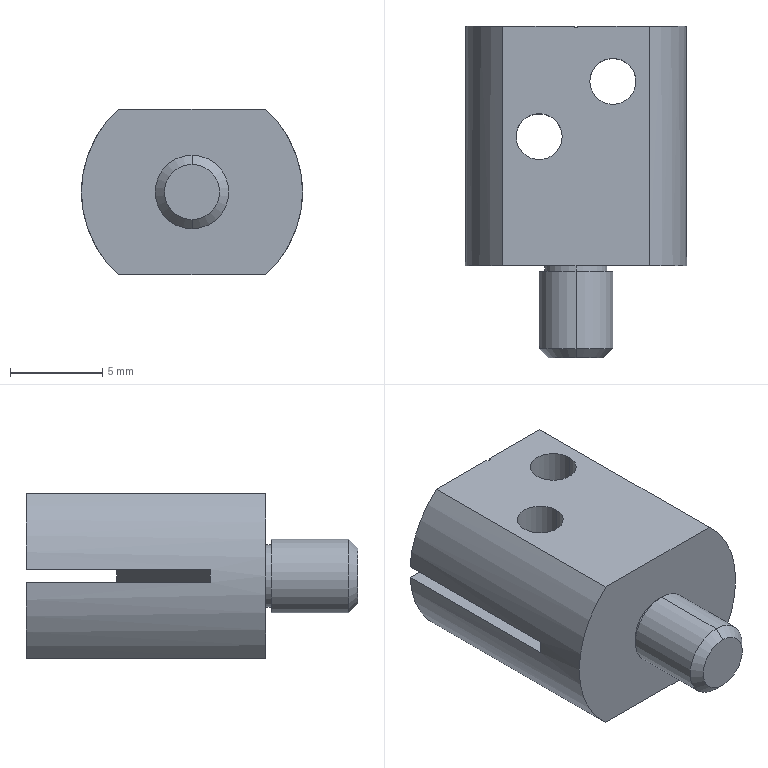Part | SolidWorks | features ICE 5, Chamfer 1, Extrusion 1, HoleWzd 1, RevCut 1 | 1 solid | 34 faces | box 12 x 18 x 9 mm | volume 1174 mm3 | plane 18 | cylinder 14 | cone 2 | commonest cylinder face diameters 2.5 x8 3.4 x2 4 x2 12 x2
STEP:
#1=CARTESIAN_POINT('',(0.75,15.,-4.5));
#2=VERTEX_POINT('',#1);
#3=CARTESIAN_POINT('',(3.25,15.,-4.5));
#4=VERTEX_POINT('',#3);
#5=CARTESIAN_POINT('',(2.,15.,-4.5));
#6=DIRECTION('',(0.,0.,1.));
#7=DIRECTION('',(1.,0.,0.));
#8=AXIS2_PLACEMENT_3D('',#5,#6,#7);
#9=CIRCLE('',#8,1.25);
#10=EDGE_CURVE('',#2,#4,#9,.T.);
#11=ORIENTED_EDGE('',*,*,#10,.F.);
#12=CARTESIAN_POINT('',(0.75,15.,-0.35));
#13=VERTEX_POINT('',#12);
#14=CARTESIAN_POINT('',(0.75,15.,4.5));
#15=DIRECTION('',(0.,0.,1.));
#16=VECTOR('',#15,1000.);
#17=LINE('',#14,#16);
#18=EDGE_CURVE('',#2,#13,#17,.T.);
#19=ORIENTED_EDGE('',*,*,#18,.T.);
#20=CARTESIAN_POINT('',(3.25,15.,-0.35));
#21=VERTEX_POINT('',#20);
#22=CARTESIAN_POINT('',(2.,15.,-0.35));
#23=DIRECTION('',(0.,0.,-1.));
#24=DIRECTION('',(-1.,0.,0.));
#25=AXIS2_PLACEMENT_3D('',#22,#23,#24);
#26=CIRCLE('',#25,1.25);
#27=EDGE_CURVE('',#21,#13,#26,.T.);
#28=ORIENTED_EDGE('',*,*,#27,.F.);
#29=CARTESIAN_POINT('',(3.25,15.,4.5));
#30=DIRECTION('',(0.,0.,1.));
#31=VECTOR('',#30,1000.);
#32=LINE('',#29,#31);
#33=EDGE_CURVE('',#4,#21,#32,.T.);
#34=ORIENTED_EDGE('',*,*,#33,.F.);
#35=EDGE_LOOP('',(#11,#19,#28,#34));
#36=FACE_OUTER_BOUND('',#35,.T.);
#37=CARTESIAN_POINT('',(2.,15.,4.5));
#38=DIRECTION('',(0.,0.,1.));
#39=DIRECTION('',(1.,0.,0.));
#40=AXIS2_PLACEMENT_3D('',#37,#38,#39);
#41=CYLINDRICAL_SURFACE('',#40,1.25);
#42=ADVANCED_FACE('',(#36),#41,.F.);
#43=CARTESIAN_POINT('',(3.25,15.,0.35));
#44=VERTEX_POINT('',#43);
#45=CARTESIAN_POINT('',(0.75,15.,0.35));
#46=VERTEX_POINT('',#45);
#47=CARTESIAN_POINT('',(2.,15.,0.35));
#48=DIRECTION('',(0.,0.,-1.));
#49=DIRECTION('',(-1.,0.,0.));
#50=AXIS2_PLACEMENT_3D('',#47,#48,#49);
#51=CIRCLE('',#50,1.25);
#52=EDGE_CURVE('',#44,#46,#51,.T.);
#53=ORIENTED_EDGE('',*,*,#52,.T.);
#54=CARTESIAN_POINT('',(0.75,15.,4.5));
#55=VERTEX_POINT('',#54);
#56=CARTESIAN_POINT('',(0.75,15.,4.5));
#57=DIRECTION('',(0.,0.,1.));
#58=VECTOR('',#57,1000.);
#59=LINE('',#56,#58);
#60=EDGE_CURVE('',#46,#55,#59,.T.);
#61=ORIENTED_EDGE('',*,*,#60,.T.);
#62=CARTESIAN_POINT('',(3.25,15.,4.5));
#63=VERTEX_POINT('',#62);
#64=CARTESIAN_POINT('',(2.,15.,4.5));
#65=DIRECTION('',(0.,0.,1.));
#66=DIRECTION('',(1.,0.,0.));
#67=AXIS2_PLACEMENT_3D('',#64,#65,#66);
#68=CIRCLE('',#67,1.25);
#69=EDGE_CURVE('',#55,#63,#68,.T.);
#70=ORIENTED_EDGE('',*,*,#69,.T.);
#71=CARTESIAN_POINT('',(3.25,15.,4.5));
#72=DIRECTION('',(0.,0.,1.));
#73=VECTOR('',#72,1000.);
#74=LINE('',#71,#73);
#75=EDGE_CURVE('',#44,#63,#74,.T.);
#76=ORIENTED_EDGE('',*,*,#75,.F.);
#77=EDGE_LOOP('',(#53,#61,#70,#76));
#78=FACE_OUTER_BOUND('',#77,.T.);
#79=CARTESIAN_POINT('',(2.,15.,4.5));
#80=DIRECTION('',(0.,0.,1.));
#81=DIRECTION('',(1.,0.,0.));
#82=AXIS2_PLACEMENT_3D('',#79,#80,#81);
#83=CYLINDRICAL_SURFACE('',#82,1.25);
#84=ADVANCED_FACE('',(#78),#83,.F.);
#85=CARTESIAN_POINT('',(-3.25,12.,-4.5));
#86=VERTEX_POINT('',#85);
#87=CARTESIAN_POINT('',(-0.75,12.,-4.5));
#88=VERTEX_POINT('',#87);
#89=CARTESIAN_POINT('',(-2.,12.,-4.5));
#90=DIRECTION('',(0.,0.,1.));
#91=DIRECTION('',(1.,0.,0.));
#92=AXIS2_PLACEMENT_3D('',#89,#90,#91);
#93=CIRCLE('',#92,1.25);
#94=EDGE_CURVE('',#86,#88,#93,.T.);
#95=ORIENTED_EDGE('',*,*,#94,.F.);
#96=CARTESIAN_POINT('',(-3.25,12.,-0.35));
#97=VERTEX_POINT('',#96);
#98=CARTESIAN_POINT('',(-3.25,12.,4.5));
#99=DIRECTION('',(0.,0.,1.));
#100=VECTOR('',#99,1000.);
#101=LINE('',#98,#100);
#102=EDGE_CURVE('',#86,#97,#101,.T.);
#103=ORIENTED_EDGE('',*,*,#102,.T.);
#104=CARTESIAN_POINT('',(-0.75,12.,-0.35));
#105=VERTEX_POINT('',#104);
#106=CARTESIAN_POINT('',(-2.,12.,-0.35));
#107=DIRECTION('',(0.,0.,-1.));
#108=DIRECTION('',(-1.,0.,0.));
#109=AXIS2_PLACEMENT_3D('',#106,#107,#108);
#110=CIRCLE('',#109,1.25);
#111=EDGE_CURVE('',#105,#97,#110,.T.);
#112=ORIENTED_EDGE('',*,*,#111,.F.);
#113=CARTESIAN_POINT('',(-0.75,12.,4.5));
#114=DIRECTION('',(0.,0.,1.));
#115=VECTOR('',#114,1000.);
#116=LINE('',#113,#115);
#117=EDGE_CURVE('',#88,#105,#116,.T.);
#118=ORIENTED_EDGE('',*,*,#117,.F.);
#119=EDGE_LOOP('',(#95,#103,#112,#118));
#120=FACE_OUTER_BOUND('',#119,.T.);
#121=CARTESIAN_POINT('',(-2.,12.,4.5));
#122=DIRECTION('',(0.,0.,1.));
#123=DIRECTION('',(1.,0.,0.));
#124=AXIS2_PLACEMENT_3D('',#121,#122,#123);
#125=CYLINDRICAL_SURFACE('',#124,1.25);
#126=ADVANCED_FACE('',(#120),#125,.F.);
#127=CARTESIAN_POINT('',(-0.75,12.,0.35));
#128=VERTEX_POINT('',#127);
#129=CARTESIAN_POINT('',(-3.25,12.,0.35));
#130=VERTEX_POINT('',#129);
#131=CARTESIAN_POINT('',(-2.,12.,0.35));
#132=DIRECTION('',(0.,0.,-1.));
#133=DIRECTION('',(-1.,0.,0.));
#134=AXIS2_PLACEMENT_3D('',#131,#132,#133);
#135=CIRCLE('',#134,1.25);
#136=EDGE_CURVE('',#128,#130,#135,.T.);
#137=ORIENTED_EDGE('',*,*,#136,.T.);
#138=CARTESIAN_POINT('',(-3.25,12.,4.5));
#139=VERTEX_POINT('',#138);
#140=CARTESIAN_POINT('',(-3.25,12.,4.5));
#141=DIRECTION('',(0.,0.,1.));
#142=VECTOR('',#141,1000.);
#143=LINE('',#140,#142);
#144=EDGE_CURVE('',#130,#139,#143,.T.);
#145=ORIENTED_EDGE('',*,*,#144,.T.);
#146=CARTESIAN_POINT('',(-0.75,12.,4.5));
#147=VERTEX_POINT('',#146);
#148=CARTESIAN_POINT('',(-2.,12.,4.5));
#149=DIRECTION('',(0.,0.,1.));
#150=DIRECTION('',(1.,0.,0.));
#151=AXIS2_PLACEMENT_3D('',#148,#149,#150);
#152=CIRCLE('',#151,1.25);
#153=EDGE_CURVE('',#139,#147,#152,.T.);
#154=ORIENTED_EDGE('',*,*,#153,.T.);
#155=CARTESIAN_POINT('',(-0.75,12.,4.5));
#156=DIRECTION('',(0.,0.,1.));
#157=VECTOR('',#156,1000.);
#158=LINE('',#155,#157);
#159=EDGE_CURVE('',#128,#147,#158,.T.);
#160=ORIENTED_EDGE('',*,*,#159,.F.);
#161=EDGE_LOOP('',(#137,#145,#154,#160));
#162=FACE_OUTER_BOUND('',#161,.T.);
#163=CARTESIAN_POINT('',(-2.,12.,4.5));
#164=DIRECTION('',(0.,0.,1.));
#165=DIRECTION('',(1.,0.,0.));
#166=AXIS2_PLACEMENT_3D('',#163,#164,#165);
#167=CYLINDRICAL_SURFACE('',#166,1.25);
#168=ADVANCED_FACE('',(#162),#167,.F.);
#169=CARTESIAN_POINT('',(0.,5.,-1.7));
#170=VERTEX_POINT('',#169);
#171=CARTESIAN_POINT('',(0.,5.,1.7));
#172=VERTEX_POINT('',#171);
#173=CARTESIAN_POINT('',(0.,5.,0.));
#174=DIRECTION('',(0.,-1.,0.));
#175=DIRECTION('',(0.,0.,-1.));
#176=AXIS2_PLACEMENT_3D('',#173,#174,#175);
#177=CIRCLE('',#176,1.7);
#178=EDGE_CURVE('',#170,#172,#177,.T.);
#179=ORIENTED_EDGE('',*,*,#178,.T.);
#180=CARTESIAN_POINT('',(0.,4.7,1.7));
#181=VERTEX_POINT('',#180);
#182=CARTESIAN_POINT('',(0.,0.,1.7));
#183=DIRECTION('',(0.,-1.,0.));
#184=VECTOR('',#183,1000.);
#185=LINE('',#182,#184);
#186=EDGE_CURVE('',#172,#181,#185,.T.);
#187=ORIENTED_EDGE('',*,*,#186,.T.);
#188=CARTESIAN_POINT('',(0.,4.7,-1.7));
#189=VERTEX_POINT('',#188);
#190=CARTESIAN_POINT('',(0.,4.7,0.));
#191=DIRECTION('',(0.,-1.,0.));
#192=DIRECTION('',(0.,0.,-1.));
#193=AXIS2_PLACEMENT_3D('',#190,#191,#192);
#194=CIRCLE('',#193,1.7);
#195=EDGE_CURVE('',#189,#181,#194,.T.);
#196=ORIENTED_EDGE('',*,*,#195,.F.);
#197=CARTESIAN_POINT('',(0.,0.,-1.7));
#198=DIRECTION('',(0.,-1.,0.));
#199=VECTOR('',#198,1000.);
#200=LINE('',#197,#199);
#201=EDGE_CURVE('',#170,#189,#200,.T.);
#202=ORIENTED_EDGE('',*,*,#201,.F.);
#203=EDGE_LOOP('',(#179,#187,#196,#202));
#204=FACE_OUTER_BOUND('',#203,.T.);
#205=CARTESIAN_POINT('',(0.,0.,0.));
#206=DIRECTION('',(0.,-1.,0.));
#207=DIRECTION('',(0.,0.,-1.));
#208=AXIS2_PLACEMENT_3D('',#205,#206,#207);
#209=CYLINDRICAL_SURFACE('',#208,1.7);
#210=ADVANCED_FACE('',(#204),#209,.T.);
#211=CARTESIAN_POINT('',(0.,0.,-1.5));
#212=VERTEX_POINT('',#211);
#213=CARTESIAN_POINT('',(0.,0.,1.5));
#214=VERTEX_POINT('',#213);
#215=CARTESIAN_POINT('',(0.,0.,0.));
#216=DIRECTION('',(0.,-1.,0.));
#217=DIRECTION('',(0.,0.,1.));
#218=AXIS2_PLACEMENT_3D('',#215,#216,#217);
#219=CIRCLE('',#218,1.5);
#220=EDGE_CURVE('',#212,#214,#219,.T.);
#221=ORIENTED_EDGE('',*,*,#220,.F.);
#222=CARTESIAN_POINT('',(0.,0.5,-2.));
#223=VERTEX_POINT('',#222);
#224=CARTESIAN_POINT('',(0.,0.,-1.5));
#225=DIRECTION('',(0.,0.7071,-0.7071));
#226=VECTOR('',#225,1000.);
#227=LINE('',#224,#226);
#228=EDGE_CURVE('',#212,#223,#227,.T.);
#229=ORIENTED_EDGE('',*,*,#228,.T.);
#230=CARTESIAN_POINT('',(0.,0.5,2.));
#231=VERTEX_POINT('',#230);
#232=CARTESIAN_POINT('',(0.,0.5,0.));
#233=DIRECTION('',(0.,1.,0.));
#234=DIRECTION('',(0.,0.,1.));
#235=AXIS2_PLACEMENT_3D('',#232,#233,#234);
#236=CIRCLE('',#235,2.);
#237=EDGE_CURVE('',#231,#223,#236,.T.);
#238=ORIENTED_EDGE('',*,*,#237,.F.);
#239=CARTESIAN_POINT('',(0.,0.,1.5));
#240=DIRECTION('',(0.,0.7071,0.7071));
#241=VECTOR('',#240,1000.);
#242=LINE('',#239,#241);
#243=EDGE_CURVE('',#214,#231,#242,.T.);
#244=ORIENTED_EDGE('',*,*,#243,.F.);
#245=EDGE_LOOP('',(#221,#229,#238,#244));
#246=FACE_OUTER_BOUND('',#245,.T.);
#247=CARTESIAN_POINT('',(0.,0.,0.));
#248=DIRECTION('',(0.,1.,0.));
#249=DIRECTION('',(0.,0.,1.));
#250=AXIS2_PLACEMENT_3D('',#247,#248,#249);
#251=CONICAL_SURFACE('',#250,1.5,0.7854);
#252=ADVANCED_FACE('',(#246),#251,.T.);
#253=CARTESIAN_POINT('',(0.,4.7,-2.));
#254=VERTEX_POINT('',#253);
#255=CARTESIAN_POINT('',(0.,4.7,2.));
#256=VERTEX_POINT('',#255);
#257=CARTESIAN_POINT('',(0.,4.7,0.));
#258=DIRECTION('',(0.,-1.,0.));
#259=DIRECTION('',(0.,0.,-1.));
#260=AXIS2_PLACEMENT_3D('',#257,#258,#259);
#261=CIRCLE('',#260,2.);
#262=EDGE_CURVE('',#254,#256,#261,.T.);
#263=ORIENTED_EDGE('',*,*,#262,.T.);
#264=CARTESIAN_POINT('',(0.,5.,2.));
#265=DIRECTION('',(0.,-1.,0.));
#266=VECTOR('',#265,1000.);
#267=LINE('',#264,#266);
#268=EDGE_CURVE('',#256,#231,#267,.T.);
#269=ORIENTED_EDGE('',*,*,#268,.T.);
#270=ORIENTED_EDGE('',*,*,#237,.T.);
#271=CARTESIAN_POINT('',(0.,5.,-2.));
#272=DIRECTION('',(0.,-1.,0.));
#273=VECTOR('',#272,1000.);
#274=LINE('',#271,#273);
#275=EDGE_CURVE('',#254,#223,#274,.T.);
#276=ORIENTED_EDGE('',*,*,#275,.F.);
#277=EDGE_LOOP('',(#263,#269,#270,#276));
#278=FACE_OUTER_BOUND('',#277,.T.);
#279=CARTESIAN_POINT('',(0.,5.,0.));
#280=DIRECTION('',(0.,-1.,0.));
#281=DIRECTION('',(0.,0.,-1.));
#282=AXIS2_PLACEMENT_3D('',#279,#280,#281);
#283=CYLINDRICAL_SURFACE('',#282,2.);
#284=ADVANCED_FACE('',(#278),#283,.T.);
#285=CARTESIAN_POINT('',(0.1,18.,4.5));
#286=VERTEX_POINT('',#285);
#287=CARTESIAN_POINT('',(0.1,18.,0.35));
#288=VERTEX_POINT('',#287);
#289=CARTESIAN_POINT('',(0.1,18.,4.5));
#290=DIRECTION('',(0.,0.,-1.));
#291=VECTOR('',#290,1000.);
#292=LINE('',#289,#291);
#293=EDGE_CURVE('',#286,#288,#292,.T.);
#294=ORIENTED_EDGE('',*,*,#293,.F.);
#295=CARTESIAN_POINT('',(3.969,18.,4.5));
#296=VERTEX_POINT('',#295);
#297=CARTESIAN_POINT('',(-6.382,18.,4.5));
#298=DIRECTION('',(1.,0.,0.));
#299=VECTOR('',#298,1000.);
#300=LINE('',#297,#299);
#301=EDGE_CURVE('',#286,#296,#300,.T.);
#302=ORIENTED_EDGE('',*,*,#301,.T.);
#303=CARTESIAN_POINT('',(5.99,18.,0.35));
#304=VERTEX_POINT('',#303);
#305=CARTESIAN_POINT('',(0.,18.,0.));
#306=DIRECTION('',(0.,1.,0.));
#307=DIRECTION('',(0.,0.,1.));
#308=AXIS2_PLACEMENT_3D('',#305,#306,#307);
#309=CIRCLE('',#308,6.);
#310=EDGE_CURVE('',#296,#304,#309,.T.);
#311=ORIENTED_EDGE('',*,*,#310,.T.);
#312=CARTESIAN_POINT('',(0.,18.,0.35));
#313=DIRECTION('',(-1.,0.,0.));
#314=VECTOR('',#313,1000.);
#315=LINE('',#312,#314);
#316=EDGE_CURVE('',#304,#288,#315,.T.);
#317=ORIENTED_EDGE('',*,*,#316,.T.);
#318=EDGE_LOOP('',(#294,#302,#311,#317));
#319=FACE_OUTER_BOUND('',#318,.T.);
#320=CARTESIAN_POINT('',(0.,18.,0.));
#321=DIRECTION('',(0.,1.,0.));
#322=DIRECTION('',(0.,0.,1.));
#323=AXIS2_PLACEMENT_3D('',#320,#321,#322);
#324=PLANE('',#323);
#325=ADVANCED_FACE('',(#319),#324,.T.);
#326=CARTESIAN_POINT('',(0.1,18.,-0.35));
#327=VERTEX_POINT('',#326);
#328=CARTESIAN_POINT('',(0.1,18.,-4.5));
#329=VERTEX_POINT('',#328);
#330=CARTESIAN_POINT('',(0.1,18.,4.5));
#331=DIRECTION('',(0.,0.,-1.));
#332=VECTOR('',#331,1000.);
#333=LINE('',#330,#332);
#334=EDGE_CURVE('',#327,#329,#333,.T.);
#335=ORIENTED_EDGE('',*,*,#334,.F.);
#336=CARTESIAN_POINT('',(5.99,18.,-0.35));
#337=VERTEX_POINT('',#336);
#338=CARTESIAN_POINT('',(0.,18.,-0.35));
#339=DIRECTION('',(-1.,0.,0.));
#340=VECTOR('',#339,1000.);
#341=LINE('',#338,#340);
#342=EDGE_CURVE('',#337,#327,#341,.T.);
#343=ORIENTED_EDGE('',*,*,#342,.F.);
#344=CARTESIAN_POINT('',(3.969,18.,-4.5));
#345=VERTEX_POINT('',#344);
#346=CARTESIAN_POINT('',(0.,18.,0.));
#347=DIRECTION('',(0.,1.,0.));
#348=DIRECTION('',(0.,0.,1.));
#349=AXIS2_PLACEMENT_3D('',#346,#347,#348);
#350=CIRCLE('',#349,6.);
#351=EDGE_CURVE('',#337,#345,#350,.T.);
#352=ORIENTED_EDGE('',*,*,#351,.T.);
#353=CARTESIAN_POINT('',(-6.382,18.,-4.5));
#354=DIRECTION('',(-1.,0.,0.));
#355=VECTOR('',#354,1000.);
#356=LINE('',#353,#355);
#357=EDGE_CURVE('',#345,#329,#356,.T.);
#358=ORIENTED_EDGE('',*,*,#357,.T.);
#359=EDGE_LOOP('',(#335,#343,#352,#358));
#360=FACE_OUTER_BOUND('',#359,.T.);
#361=CARTESIAN_POINT('',(0.,18.,0.));
#362=DIRECTION('',(0.,1.,0.));
#363=DIRECTION('',(0.,0.,1.));
#364=AXIS2_PLACEMENT_3D('',#361,#362,#363);
#365=PLANE('',#364);
#366=ADVANCED_FACE('',(#360),#365,.T.);
#367=CARTESIAN_POINT('',(-0.1,18.,0.35));
#368=VERTEX_POINT('',#367);
#369=CARTESIAN_POINT('',(-0.1,18.,4.5));
#370=VERTEX_POINT('',#369);
#371=CARTESIAN_POINT('',(-0.1,18.,4.5));
#372=DIRECTION('',(0.,0.,1.));
#373=VECTOR('',#372,1000.);
#374=LINE('',#371,#373);
#375=EDGE_CURVE('',#368,#370,#374,.T.);
#376=ORIENTED_EDGE('',*,*,#375,.F.);
#377=CARTESIAN_POINT('',(-5.99,18.,0.35));
#378=VERTEX_POINT('',#377);
#379=CARTESIAN_POINT('',(0.,18.,0.35));
#380=DIRECTION('',(-1.,0.,0.));
#381=VECTOR('',#380,1000.);
#382=LINE('',#379,#381);
#383=EDGE_CURVE('',#368,#378,#382,.T.);
#384=ORIENTED_EDGE('',*,*,#383,.T.);
#385=CARTESIAN_POINT('',(-3.969,18.,4.5));
#386=VERTEX_POINT('',#385);
#387=CARTESIAN_POINT('',(0.,18.,0.));
#388=DIRECTION('',(0.,1.,0.));
#389=DIRECTION('',(0.,0.,1.));
#390=AXIS2_PLACEMENT_3D('',#387,#388,#389);
#391=CIRCLE('',#390,6.);
#392=EDGE_CURVE('',#378,#386,#391,.T.);
#393=ORIENTED_EDGE('',*,*,#392,.T.);
#394=CARTESIAN_POINT('',(-6.382,18.,4.5));
#395=DIRECTION('',(1.,0.,0.));
#396=VECTOR('',#395,1000.);
#397=LINE('',#394,#396);
#398=EDGE_CURVE('',#386,#370,#397,.T.);
#399=ORIENTED_EDGE('',*,*,#398,.T.);
#400=EDGE_LOOP('',(#376,#384,#393,#399));
#401=FACE_OUTER_BOUND('',#400,.T.);
#402=CARTESIAN_POINT('',(0.,18.,0.));
#403=DIRECTION('',(0.,1.,0.));
#404=DIRECTION('',(0.,0.,1.));
#405=AXIS2_PLACEMENT_3D('',#402,#403,#404);
#406=PLANE('',#405);
#407=ADVANCED_FACE('',(#401),#406,.T.);
#408=CARTESIAN_POINT('',(-0.1,18.,-4.5));
#409=VERTEX_POINT('',#408);
#410=CARTESIAN_POINT('',(-0.1,18.,-0.35));
#411=VERTEX_POINT('',#410);
#412=CARTESIAN_POINT('',(-0.1,18.,4.5));
#413=DIRECTION('',(0.,0.,1.));
#414=VECTOR('',#413,1000.);
#415=LINE('',#412,#414);
#416=EDGE_CURVE('',#409,#411,#415,.T.);
#417=ORIENTED_EDGE('',*,*,#416,.F.);
#418=CARTESIAN_POINT('',(-3.969,18.,-4.5));
#419=VERTEX_POINT('',#418);
#420=CARTESIAN_POINT('',(-6.382,18.,-4.5));
#421=DIRECTION('',(-1.,0.,0.));
#422=VECTOR('',#421,1000.);
#423=LINE('',#420,#422);
#424=EDGE_CURVE('',#409,#419,#423,.T.);
#425=ORIENTED_EDGE('',*,*,#424,.T.);
#426=CARTESIAN_POINT('',(-5.99,18.,-0.35));
#427=VERTEX_POINT('',#426);
#428=CARTESIAN_POINT('',(0.,18.,0.));
#429=DIRECTION('',(0.,1.,0.));
#430=DIRECTION('',(0.,0.,1.));
#431=AXIS2_PLACEMENT_3D('',#428,#429,#430);
#432=CIRCLE('',#431,6.);
#433=EDGE_CURVE('',#419,#427,#432,.T.);
#434=ORIENTED_EDGE('',*,*,#433,.T.);
#435=CARTESIAN_POINT('',(0.,18.,-0.35));
#436=DIRECTION('',(-1.,0.,0.));
#437=VECTOR('',#436,1000.);
#438=LINE('',#435,#437);
#439=EDGE_CURVE('',#411,#427,#438,.T.);
#440=ORIENTED_EDGE('',*,*,#439,.F.);
#441=EDGE_LOOP('',(#417,#425,#434,#440));
#442=FACE_OUTER_BOUND('',#441,.T.);
#443=CARTESIAN_POINT('',(0.,18.,0.));
#444=DIRECTION('',(0.,1.,0.));
#445=DIRECTION('',(0.,0.,1.));
#446=AXIS2_PLACEMENT_3D('',#443,#444,#445);
#447=PLANE('',#446);
#448=ADVANCED_FACE('',(#442),#447,.T.);
#449=CARTESIAN_POINT('',(-3.969,5.,4.5));
#450=VERTEX_POINT('',#449);
#451=CARTESIAN_POINT('',(-3.969,18.,4.5));
#452=DIRECTION('',(0.,-1.,0.));
#453=VECTOR('',#452,1000.);
#454=LINE('',#451,#453);
#455=EDGE_CURVE('',#386,#450,#454,.T.);
#456=ORIENTED_EDGE('',*,*,#455,.F.);
#457=ORIENTED_EDGE('',*,*,#392,.F.);
#458=CARTESIAN_POINT('',(-5.99,8.004,0.35));
#459=VERTEX_POINT('',#458);
#460=CARTESIAN_POINT('',(-5.99,18.,0.35));
#461=DIRECTION('',(0.,1.,0.));
#462=VECTOR('',#461,1000.);
#463=LINE('',#460,#462);
#464=EDGE_CURVE('',#459,#378,#463,.T.);
#465=ORIENTED_EDGE('',*,*,#464,.F.);
#466=CARTESIAN_POINT('',(-5.99,8.004,-0.35));
#467=VERTEX_POINT('',#466);
#468=CARTESIAN_POINT('',(-5.99,8.004,0.35));
#469=CARTESIAN_POINT('',(-6.003,7.999,0.1168));
#470=CARTESIAN_POINT('',(-6.003,7.999,-0.1168));
#471=CARTESIAN_POINT('',(-5.99,8.004,-0.35));
#472=(BOUNDED_CURVE()B_SPLINE_CURVE(3,(#468,#469,#470,#471),.UNSPECIFIED.,.F.,.T.)B_SPLINE_CURVE_WITH_KNOTS((4,4),(6.225,6.342),.UNSPECIFIED.)CURVE()GEOMETRIC_REPRESENTATION_ITEM()RATIONAL_B_SPLINE_CURVE((1.,0.9989,0.9989,1.))REPRESENTATION_ITEM(''));
#473=EDGE_CURVE('',#459,#467,#472,.T.);
#474=ORIENTED_EDGE('',*,*,#473,.T.);
#475=CARTESIAN_POINT('',(-5.99,18.,-0.35));
#476=DIRECTION('',(0.,1.,0.));
#477=VECTOR('',#476,1000.);
#478=LINE('',#475,#477);
#479=EDGE_CURVE('',#467,#427,#478,.T.);
#480=ORIENTED_EDGE('',*,*,#479,.T.);
#481=ORIENTED_EDGE('',*,*,#433,.F.);
#482=CARTESIAN_POINT('',(-3.969,5.,-4.5));
#483=VERTEX_POINT('',#482);
#484=CARTESIAN_POINT('',(-3.969,18.,-4.5));
#485=DIRECTION('',(0.,1.,0.));
#486=VECTOR('',#485,1000.);
#487=LINE('',#484,#486);
#488=EDGE_CURVE('',#483,#419,#487,.T.);
#489=ORIENTED_EDGE('',*,*,#488,.F.);
#490=CARTESIAN_POINT('',(0.,5.,0.));
#491=DIRECTION('',(0.,-1.,0.));
#492=DIRECTION('',(0.,0.,-1.));
#493=AXIS2_PLACEMENT_3D('',#490,#491,#492);
#494=CIRCLE('',#493,6.);
#495=EDGE_CURVE('',#450,#483,#494,.T.);
#496=ORIENTED_EDGE('',*,*,#495,.F.);
#497=EDGE_LOOP('',(#456,#457,#465,#474,#480,#481,#489,#496));
#498=FACE_OUTER_BOUND('',#497,.T.);
#499=CARTESIAN_POINT('',(0.,18.,0.));
#500=DIRECTION('',(0.,-1.,0.));
#501=DIRECTION('',(0.,0.,-1.));
#502=AXIS2_PLACEMENT_3D('',#499,#500,#501);
#503=CYLINDRICAL_SURFACE('',#502,6.);
#504=ADVANCED_FACE('',(#498),#503,.T.);
#505=CARTESIAN_POINT('',(3.969,5.,4.5));
#506=VERTEX_POINT('',#505);
#507=CARTESIAN_POINT('',(3.969,18.,4.5));
#508=DIRECTION('',(0.,1.,0.));
#509=VECTOR('',#508,1000.);
#510=LINE('',#507,#509);
#511=EDGE_CURVE('',#506,#296,#510,.T.);
#512=ORIENTED_EDGE('',*,*,#511,.F.);
#513=CARTESIAN_POINT('',(3.969,5.,-4.5));
#514=VERTEX_POINT('',#513);
#515=CARTESIAN_POINT('',(0.,5.,0.));
#516=DIRECTION('',(0.,-1.,0.));
#517=DIRECTION('',(0.,0.,-1.));
#518=AXIS2_PLACEMENT_3D('',#515,#516,#517);
#519=CIRCLE('',#518,6.);
#520=EDGE_CURVE('',#514,#506,#519,.T.);
#521=ORIENTED_EDGE('',*,*,#520,.F.);
#522=CARTESIAN_POINT('',(3.969,18.,-4.5));
#523=DIRECTION('',(0.,-1.,0.));
#524=VECTOR('',#523,1000.);
#525=LINE('',#522,#524);
#526=EDGE_CURVE('',#345,#514,#525,.T.);
#527=ORIENTED_EDGE('',*,*,#526,.F.);
#528=ORIENTED_EDGE('',*,*,#351,.F.);
#529=CARTESIAN_POINT('',(5.99,13.089,-0.35));
#530=VERTEX_POINT('',#529);
#531=CARTESIAN_POINT('',(5.99,18.,-0.35));
#532=DIRECTION('',(0.,-1.,0.));
#533=VECTOR('',#532,1000.);
#534=LINE('',#531,#533);
#535=EDGE_CURVE('',#337,#530,#534,.T.);
#536=ORIENTED_EDGE('',*,*,#535,.T.);
#537=CARTESIAN_POINT('',(5.99,13.089,0.35));
#538=VERTEX_POINT('',#537);
#539=CARTESIAN_POINT('',(5.99,13.089,-0.35));
#540=CARTESIAN_POINT('',(6.003,13.095,-0.1168));
#541=CARTESIAN_POINT('',(6.003,13.095,0.1168));
#542=CARTESIAN_POINT('',(5.99,13.089,0.35));
#543=(BOUNDED_CURVE()B_SPLINE_CURVE(3,(#539,#540,#541,#542),.UNSPECIFIED.,.F.,.T.)B_SPLINE_CURVE_WITH_KNOTS((4,4),(3.083,3.2),.UNSPECIFIED.)CURVE()GEOMETRIC_REPRESENTATION_ITEM()RATIONAL_B_SPLINE_CURVE((1.,0.9989,0.9989,1.))REPRESENTATION_ITEM(''));
#544=EDGE_CURVE('',#530,#538,#543,.T.);
#545=ORIENTED_EDGE('',*,*,#544,.T.);
#546=CARTESIAN_POINT('',(5.99,18.,0.35));
#547=DIRECTION('',(0.,-1.,0.));
#548=VECTOR('',#547,1000.);
#549=LINE('',#546,#548);
#550=EDGE_CURVE('',#304,#538,#549,.T.);
#551=ORIENTED_EDGE('',*,*,#550,.F.);
#552=ORIENTED_EDGE('',*,*,#310,.F.);
#553=EDGE_LOOP('',(#512,#521,#527,#528,#536,#545,#551,#552));
#554=FACE_OUTER_BOUND('',#553,.T.);
#555=CARTESIAN_POINT('',(0.,18.,0.));
#556=DIRECTION('',(0.,-1.,0.));
#557=DIRECTION('',(0.,0.,-1.));
#558=AXIS2_PLACEMENT_3D('',#555,#556,#557);
#559=CYLINDRICAL_SURFACE('',#558,6.);
#560=ADVANCED_FACE('',(#554),#559,.T.);
#561=ORIENTED_EDGE('',*,*,#178,.F.);
#562=CARTESIAN_POINT('',(0.,5.,0.));
#563=DIRECTION('',(0.,-1.,0.));
#564=DIRECTION('',(0.,0.,-1.));
#565=AXIS2_PLACEMENT_3D('',#562,#563,#564);
#566=CIRCLE('',#565,1.7);
#567=EDGE_CURVE('',#172,#170,#566,.T.);
#568=ORIENTED_EDGE('',*,*,#567,.F.);
#569=EDGE_LOOP('',(#561,#568));
#570=FACE_BOUND('',#569,.T.);
#571=ORIENTED_EDGE('',*,*,#520,.T.);
#572=CARTESIAN_POINT('',(0.,5.,4.5));
#573=DIRECTION('',(-1.,0.,0.));
#574=VECTOR('',#573,1000.);
#575=LINE('',#572,#574);
#576=EDGE_CURVE('',#506,#450,#575,.T.);
#577=ORIENTED_EDGE('',*,*,#576,.T.);
#578=ORIENTED_EDGE('',*,*,#495,.T.);
#579=CARTESIAN_POINT('',(0.,5.,-4.5));
#580=DIRECTION('',(1.,0.,0.));
#581=VECTOR('',#580,1000.);
#582=LINE('',#579,#581);
#583=EDGE_CURVE('',#483,#514,#582,.T.);
#584=ORIENTED_EDGE('',*,*,#583,.T.);
#585=EDGE_LOOP('',(#571,#577,#578,#584));
#586=FACE_OUTER_BOUND('',#585,.T.);
#587=CARTESIAN_POINT('',(0.,5.,0.));
#588=DIRECTION('',(0.,-1.,0.));
#589=DIRECTION('',(0.,0.,-1.));
#590=AXIS2_PLACEMENT_3D('',#587,#588,#589);
#591=PLANE('',#590);
#592=ADVANCED_FACE('',(#570,#586),#591,.T.);
#593=ORIENTED_EDGE('',*,*,#268,.F.);
#594=CARTESIAN_POINT('',(0.,4.7,0.));
#595=DIRECTION('',(0.,-1.,0.));
#596=DIRECTION('',(0.,0.,-1.));
#597=AXIS2_PLACEMENT_3D('',#594,#595,#596);
#598=CIRCLE('',#597,2.);
#599=EDGE_CURVE('',#256,#254,#598,.T.);
#600=ORIENTED_EDGE('',*,*,#599,.T.);
#601=ORIENTED_EDGE('',*,*,#275,.T.);
#602=CARTESIAN_POINT('',(0.,0.5,0.));
#603=DIRECTION('',(0.,1.,0.));
#604=DIRECTION('',(0.,0.,1.));
#605=AXIS2_PLACEMENT_3D('',#602,#603,#604);
#606=CIRCLE('',#605,2.);
#607=EDGE_CURVE('',#223,#231,#606,.T.);
#608=ORIENTED_EDGE('',*,*,#607,.T.);
#609=EDGE_LOOP('',(#593,#600,#601,#608));
#610=FACE_OUTER_BOUND('',#609,.T.);
#611=CARTESIAN_POINT('',(0.,5.,0.));
#612=DIRECTION('',(0.,-1.,0.));
#613=DIRECTION('',(0.,0.,-1.));
#614=AXIS2_PLACEMENT_3D('',#611,#612,#613);
#615=CYLINDRICAL_SURFACE('',#614,2.);
#616=ADVANCED_FACE('',(#610),#615,.T.);
#617=CARTESIAN_POINT('',(0.,0.,0.));
#618=DIRECTION('',(0.,-1.,0.));
#619=DIRECTION('',(0.,0.,1.));
#620=AXIS2_PLACEMENT_3D('',#617,#618,#619);
#621=CIRCLE('',#620,1.5);
#622=EDGE_CURVE('',#214,#212,#621,.T.);
#623=ORIENTED_EDGE('',*,*,#622,.T.);
#624=ORIENTED_EDGE('',*,*,#220,.T.);
#625=EDGE_LOOP('',(#623,#624));
#626=FACE_OUTER_BOUND('',#625,.T.);
#627=CARTESIAN_POINT('',(0.,0.,0.));
#628=DIRECTION('',(0.,1.,0.));
#629=DIRECTION('',(0.,0.,1.));
#630=AXIS2_PLACEMENT_3D('',#627,#628,#629);
#631=PLANE('',#630);
#632=ADVANCED_FACE('',(#626),#631,.F.);
#633=ORIENTED_EDGE('',*,*,#228,.F.);
#634=ORIENTED_EDGE('',*,*,#622,.F.);
#635=ORIENTED_EDGE('',*,*,#243,.T.);
#636=ORIENTED_EDGE('',*,*,#607,.F.);
#637=EDGE_LOOP('',(#633,#634,#635,#636));
#638=FACE_OUTER_BOUND('',#637,.T.);
#639=CARTESIAN_POINT('',(0.,0.,0.));
#640=DIRECTION('',(0.,1.,0.));
#641=DIRECTION('',(0.,0.,1.));
#642=AXIS2_PLACEMENT_3D('',#639,#640,#641);
#643=CONICAL_SURFACE('',#642,1.5,0.7854);
#644=ADVANCED_FACE('',(#638),#643,.T.);
#645=ORIENTED_EDGE('',*,*,#262,.F.);
#646=ORIENTED_EDGE('',*,*,#599,.F.);
#647=EDGE_LOOP('',(#645,#646));
#648=FACE_OUTER_BOUND('',#647,.T.);
#649=ORIENTED_EDGE('',*,*,#195,.T.);
#650=CARTESIAN_POINT('',(0.,4.7,0.));
#651=DIRECTION('',(0.,-1.,0.));
#652=DIRECTION('',(0.,0.,-1.));
#653=AXIS2_PLACEMENT_3D('',#650,#651,#652);
#654=CIRCLE('',#653,1.7);
#655=EDGE_CURVE('',#181,#189,#654,.T.);
#656=ORIENTED_EDGE('',*,*,#655,.T.);
#657=EDGE_LOOP('',(#649,#656));
#658=FACE_BOUND('',#657,.T.);
#659=CARTESIAN_POINT('',(2.,4.7,0.));
#660=DIRECTION('',(0.,-1.,0.));
#661=DIRECTION('',(0.,0.,-1.));
#662=AXIS2_PLACEMENT_3D('',#659,#660,#661);
#663=PLANE('',#662);
#664=ADVANCED_FACE('',(#648,#658),#663,.F.);
#665=ORIENTED_EDGE('',*,*,#186,.F.);
#666=ORIENTED_EDGE('',*,*,#567,.T.);
#667=ORIENTED_EDGE('',*,*,#201,.T.);
#668=ORIENTED_EDGE('',*,*,#655,.F.);
#669=EDGE_LOOP('',(#665,#666,#667,#668));
#670=FACE_OUTER_BOUND('',#669,.T.);
#671=CARTESIAN_POINT('',(0.,0.,0.));
#672=DIRECTION('',(0.,-1.,0.));
#673=DIRECTION('',(0.,0.,-1.));
#674=AXIS2_PLACEMENT_3D('',#671,#672,#673);
#675=CYLINDRICAL_SURFACE('',#674,1.7);
#676=ADVANCED_FACE('',(#670),#675,.T.);
#677=CARTESIAN_POINT('',(0.1,17.9,0.35));
#678=VERTEX_POINT('',#677);
#679=CARTESIAN_POINT('',(0.1,0.,0.35));
#680=DIRECTION('',(0.,-1.,0.));
#681=VECTOR('',#680,1000.);
#682=LINE('',#679,#681);
#683=EDGE_CURVE('',#288,#678,#682,.T.);
#684=ORIENTED_EDGE('',*,*,#683,.F.);
#685=ORIENTED_EDGE('',*,*,#316,.F.);
#686=ORIENTED_EDGE('',*,*,#550,.T.);
#687=CARTESIAN_POINT('',(-6.,8.,0.35));
#688=DIRECTION('',(0.9205,0.3907,0.));
#689=VECTOR('',#688,1000.);
#690=LINE('',#687,#689);
#691=EDGE_CURVE('',#459,#538,#690,.T.);
#692=ORIENTED_EDGE('',*,*,#691,.F.);
#693=ORIENTED_EDGE('',*,*,#464,.T.);
#694=ORIENTED_EDGE('',*,*,#383,.F.);
#695=CARTESIAN_POINT('',(-0.1,17.9,0.35));
#696=VERTEX_POINT('',#695);
#697=CARTESIAN_POINT('',(-0.1,0.,0.35));
#698=DIRECTION('',(0.,1.,0.));
#699=VECTOR('',#698,1000.);
#700=LINE('',#697,#699);
#701=EDGE_CURVE('',#696,#368,#700,.T.);
#702=ORIENTED_EDGE('',*,*,#701,.F.);
#703=CARTESIAN_POINT('',(0.,17.9,0.35));
#704=DIRECTION('',(-1.,0.,0.));
#705=VECTOR('',#704,1000.);
#706=LINE('',#703,#705);
#707=EDGE_CURVE('',#678,#696,#706,.T.);
#708=ORIENTED_EDGE('',*,*,#707,.F.);
#709=EDGE_LOOP('',(#684,#685,#686,#692,#693,#694,#702,#708));
#710=FACE_OUTER_BOUND('',#709,.T.);
#711=ORIENTED_EDGE('',*,*,#52,.F.);
#712=CARTESIAN_POINT('',(2.,15.,0.35));
#713=DIRECTION('',(0.,0.,-1.));
#714=DIRECTION('',(-1.,0.,0.));
#715=AXIS2_PLACEMENT_3D('',#712,#713,#714);
#716=CIRCLE('',#715,1.25);
#717=EDGE_CURVE('',#46,#44,#716,.T.);
#718=ORIENTED_EDGE('',*,*,#717,.F.);
#719=EDGE_LOOP('',(#711,#718));
#720=FACE_BOUND('',#719,.T.);
#721=ORIENTED_EDGE('',*,*,#136,.F.);
#722=CARTESIAN_POINT('',(-2.,12.,0.35));
#723=DIRECTION('',(0.,0.,-1.));
#724=DIRECTION('',(-1.,0.,0.));
#725=AXIS2_PLACEMENT_3D('',#722,#723,#724);
#726=CIRCLE('',#725,1.25);
#727=EDGE_CURVE('',#130,#128,#726,.T.);
#728=ORIENTED_EDGE('',*,*,#727,.F.);
#729=EDGE_LOOP('',(#721,#728));
#730=FACE_BOUND('',#729,.T.);
#731=CARTESIAN_POINT('',(0.,0.,0.35));
#732=DIRECTION('',(0.,0.,-1.));
#733=DIRECTION('',(-1.,0.,0.));
#734=AXIS2_PLACEMENT_3D('',#731,#732,#733);
#735=PLANE('',#734);
#736=ADVANCED_FACE('',(#710,#720,#730),#735,.T.);
#737=CARTESIAN_POINT('',(-6.,8.,-0.35));
#738=DIRECTION('',(0.9205,0.3907,0.));
#739=VECTOR('',#738,1000.);
#740=LINE('',#737,#739);
#741=EDGE_CURVE('',#467,#530,#740,.T.);
#742=ORIENTED_EDGE('',*,*,#741,.F.);
#743=ORIENTED_EDGE('',*,*,#473,.F.);
#744=ORIENTED_EDGE('',*,*,#691,.T.);
#745=ORIENTED_EDGE('',*,*,#544,.F.);
#746=EDGE_LOOP('',(#742,#743,#744,#745));
#747=FACE_OUTER_BOUND('',#746,.T.);
#748=CARTESIAN_POINT('',(-6.,8.,-0.35));
#749=DIRECTION('',(0.3907,-0.9205,0.));
#750=DIRECTION('',(0.9205,0.3907,0.));
#751=AXIS2_PLACEMENT_3D('',#748,#749,#750);
#752=PLANE('',#751);
#753=ADVANCED_FACE('',(#747),#752,.F.);
#754=ORIENTED_EDGE('',*,*,#342,.T.);
#755=CARTESIAN_POINT('',(0.1,17.9,-0.35));
#756=VERTEX_POINT('',#755);
#757=CARTESIAN_POINT('',(0.1,0.,-0.35));
#758=DIRECTION('',(0.,-1.,0.));
#759=VECTOR('',#758,1000.);
#760=LINE('',#757,#759);
#761=EDGE_CURVE('',#327,#756,#760,.T.);
#762=ORIENTED_EDGE('',*,*,#761,.T.);
#763=CARTESIAN_POINT('',(-0.1,17.9,-0.35));
#764=VERTEX_POINT('',#763);
#765=CARTESIAN_POINT('',(0.,17.9,-0.35));
#766=DIRECTION('',(-1.,0.,0.));
#767=VECTOR('',#766,1000.);
#768=LINE('',#765,#767);
#769=EDGE_CURVE('',#756,#764,#768,.T.);
#770=ORIENTED_EDGE('',*,*,#769,.T.);
#771=CARTESIAN_POINT('',(-0.1,0.,-0.35));
#772=DIRECTION('',(0.,1.,0.));
#773=VECTOR('',#772,1000.);
#774=LINE('',#771,#773);
#775=EDGE_CURVE('',#764,#411,#774,.T.);
#776=ORIENTED_EDGE('',*,*,#775,.T.);
#777=ORIENTED_EDGE('',*,*,#439,.T.);
#778=ORIENTED_EDGE('',*,*,#479,.F.);
#779=ORIENTED_EDGE('',*,*,#741,.T.);
#780=ORIENTED_EDGE('',*,*,#535,.F.);
#781=EDGE_LOOP('',(#754,#762,#770,#776,#777,#778,#779,#780));
#782=FACE_OUTER_BOUND('',#781,.T.);
#783=ORIENTED_EDGE('',*,*,#27,.T.);
#784=CARTESIAN_POINT('',(2.,15.,-0.35));
#785=DIRECTION('',(0.,0.,-1.));
#786=DIRECTION('',(-1.,0.,0.));
#787=AXIS2_PLACEMENT_3D('',#784,#785,#786);
#788=CIRCLE('',#787,1.25);
#789=EDGE_CURVE('',#13,#21,#788,.T.);
#790=ORIENTED_EDGE('',*,*,#789,.T.);
#791=EDGE_LOOP('',(#783,#790));
#792=FACE_BOUND('',#791,.T.);
#793=ORIENTED_EDGE('',*,*,#111,.T.);
#794=CARTESIAN_POINT('',(-2.,12.,-0.35));
#795=DIRECTION('',(0.,0.,-1.));
#796=DIRECTION('',(-1.,0.,0.));
#797=AXIS2_PLACEMENT_3D('',#794,#795,#796);
#798=CIRCLE('',#797,1.25);
#799=EDGE_CURVE('',#97,#105,#798,.T.);
#800=ORIENTED_EDGE('',*,*,#799,.T.);
#801=EDGE_LOOP('',(#793,#800));
#802=FACE_BOUND('',#801,.T.);
#803=CARTESIAN_POINT('',(0.,0.,-0.35));
#804=DIRECTION('',(0.,0.,-1.));
#805=DIRECTION('',(-1.,0.,0.));
#806=AXIS2_PLACEMENT_3D('',#803,#804,#805);
#807=PLANE('',#806);
#808=ADVANCED_FACE('',(#782,#792,#802),#807,.F.);
#809=CARTESIAN_POINT('',(0.1,17.9,-4.5));
#810=VERTEX_POINT('',#809);
#811=CARTESIAN_POINT('',(0.1,17.9,-4.5));
#812=DIRECTION('',(0.,1.,0.));
#813=VECTOR('',#812,1000.);
#814=LINE('',#811,#813);
#815=EDGE_CURVE('',#810,#329,#814,.T.);
#816=ORIENTED_EDGE('',*,*,#815,.T.);
#817=ORIENTED_EDGE('',*,*,#357,.F.);
#818=ORIENTED_EDGE('',*,*,#526,.T.);
#819=ORIENTED_EDGE('',*,*,#583,.F.);
#820=ORIENTED_EDGE('',*,*,#488,.T.);
#821=ORIENTED_EDGE('',*,*,#424,.F.);
#822=CARTESIAN_POINT('',(-0.1,17.9,-4.5));
#823=VERTEX_POINT('',#822);
#824=CARTESIAN_POINT('',(-0.1,17.9,-4.5));
#825=DIRECTION('',(0.,1.,0.));
#826=VECTOR('',#825,1000.);
#827=LINE('',#824,#826);
#828=EDGE_CURVE('',#823,#409,#827,.T.);
#829=ORIENTED_EDGE('',*,*,#828,.F.);
#830=CARTESIAN_POINT('',(-0.1,17.9,-4.5));
#831=DIRECTION('',(-1.,0.,0.));
#832=VECTOR('',#831,1000.);
#833=LINE('',#830,#832);
#834=EDGE_CURVE('',#810,#823,#833,.T.);
#835=ORIENTED_EDGE('',*,*,#834,.F.);
#836=EDGE_LOOP('',(#816,#817,#818,#819,#820,#821,#829,#835));
#837=FACE_OUTER_BOUND('',#836,.T.);
#838=CARTESIAN_POINT('',(2.,15.,-4.5));
#839=DIRECTION('',(0.,0.,1.));
#840=DIRECTION('',(1.,0.,0.));
#841=AXIS2_PLACEMENT_3D('',#838,#839,#840);
#842=CIRCLE('',#841,1.25);
#843=EDGE_CURVE('',#4,#2,#842,.T.);
#844=ORIENTED_EDGE('',*,*,#843,.T.);
#845=ORIENTED_EDGE('',*,*,#10,.T.);
#846=EDGE_LOOP('',(#844,#845));
#847=FACE_BOUND('',#846,.T.);
#848=CARTESIAN_POINT('',(-2.,12.,-4.5));
#849=DIRECTION('',(0.,0.,1.));
#850=DIRECTION('',(1.,0.,0.));
#851=AXIS2_PLACEMENT_3D('',#848,#849,#850);
#852=CIRCLE('',#851,1.25);
#853=EDGE_CURVE('',#88,#86,#852,.T.);
#854=ORIENTED_EDGE('',*,*,#853,.T.);
#855=ORIENTED_EDGE('',*,*,#94,.T.);
#856=EDGE_LOOP('',(#854,#855));
#857=FACE_BOUND('',#856,.T.);
#858=CARTESIAN_POINT('',(-6.382,0.,-4.5));
#859=DIRECTION('',(0.,0.,-1.));
#860=DIRECTION('',(-1.,0.,0.));
#861=AXIS2_PLACEMENT_3D('',#858,#859,#860);
#862=PLANE('',#861);
#863=ADVANCED_FACE('',(#837,#847,#857),#862,.T.);
#864=CARTESIAN_POINT('',(0.1,17.9,4.5));
#865=VERTEX_POINT('',#864);
#866=CARTESIAN_POINT('',(0.1,17.9,4.5));
#867=DIRECTION('',(0.,1.,0.));
#868=VECTOR('',#867,1000.);
#869=LINE('',#866,#868);
#870=EDGE_CURVE('',#865,#286,#869,.T.);
#871=ORIENTED_EDGE('',*,*,#870,.F.);
#872=CARTESIAN_POINT('',(-0.1,17.9,4.5));
#873=VERTEX_POINT('',#872);
#874=CARTESIAN_POINT('',(-0.1,17.9,4.5));
#875=DIRECTION('',(1.,0.,0.));
#876=VECTOR('',#875,1000.);
#877=LINE('',#874,#876);
#878=EDGE_CURVE('',#873,#865,#877,.T.);
#879=ORIENTED_EDGE('',*,*,#878,.F.);
#880=CARTESIAN_POINT('',(-0.1,17.9,4.5));
#881=DIRECTION('',(0.,1.,0.));
#882=VECTOR('',#881,1000.);
#883=LINE('',#880,#882);
#884=EDGE_CURVE('',#873,#370,#883,.T.);
#885=ORIENTED_EDGE('',*,*,#884,.T.);
#886=ORIENTED_EDGE('',*,*,#398,.F.);
#887=ORIENTED_EDGE('',*,*,#455,.T.);
#888=ORIENTED_EDGE('',*,*,#576,.F.);
#889=ORIENTED_EDGE('',*,*,#511,.T.);
#890=ORIENTED_EDGE('',*,*,#301,.F.);
#891=EDGE_LOOP('',(#871,#879,#885,#886,#887,#888,#889,#890));
#892=FACE_OUTER_BOUND('',#891,.T.);
#893=CARTESIAN_POINT('',(2.,15.,4.5));
#894=DIRECTION('',(0.,0.,1.));
#895=DIRECTION('',(1.,0.,0.));
#896=AXIS2_PLACEMENT_3D('',#893,#894,#895);
#897=CIRCLE('',#896,1.25);
#898=EDGE_CURVE('',#63,#55,#897,.T.);
#899=ORIENTED_EDGE('',*,*,#898,.F.);
#900=ORIENTED_EDGE('',*,*,#69,.F.);
#901=EDGE_LOOP('',(#899,#900));
#902=FACE_BOUND('',#901,.T.);
#903=CARTESIAN_POINT('',(-2.,12.,4.5));
#904=DIRECTION('',(0.,0.,1.));
#905=DIRECTION('',(1.,0.,0.));
#906=AXIS2_PLACEMENT_3D('',#903,#904,#905);
#907=CIRCLE('',#906,1.25);
#908=EDGE_CURVE('',#147,#139,#907,.T.);
#909=ORIENTED_EDGE('',*,*,#908,.F.);
#910=ORIENTED_EDGE('',*,*,#153,.F.);
#911=EDGE_LOOP('',(#909,#910));
#912=FACE_BOUND('',#911,.T.);
#913=CARTESIAN_POINT('',(-6.382,0.,4.5));
#914=DIRECTION('',(0.,0.,1.));
#915=DIRECTION('',(1.,0.,0.));
#916=AXIS2_PLACEMENT_3D('',#913,#914,#915);
#917=PLANE('',#916);
#918=ADVANCED_FACE('',(#892,#902,#912),#917,.T.);
#919=ORIENTED_EDGE('',*,*,#144,.F.);
#920=ORIENTED_EDGE('',*,*,#727,.T.);
#921=ORIENTED_EDGE('',*,*,#159,.T.);
#922=ORIENTED_EDGE('',*,*,#908,.T.);
#923=EDGE_LOOP('',(#919,#920,#921,#922));
#924=FACE_OUTER_BOUND('',#923,.T.);
#925=CARTESIAN_POINT('',(-2.,12.,4.5));
#926=DIRECTION('',(0.,0.,1.));
#927=DIRECTION('',(1.,0.,0.));
#928=AXIS2_PLACEMENT_3D('',#925,#926,#927);
#929=CYLINDRICAL_SURFACE('',#928,1.25);
#930=ADVANCED_FACE('',(#924),#929,.F.);
#931=ORIENTED_EDGE('',*,*,#102,.F.);
#932=ORIENTED_EDGE('',*,*,#853,.F.);
#933=ORIENTED_EDGE('',*,*,#117,.T.);
#934=ORIENTED_EDGE('',*,*,#799,.F.);
#935=EDGE_LOOP('',(#931,#932,#933,#934));
#936=FACE_OUTER_BOUND('',#935,.T.);
#937=CARTESIAN_POINT('',(-2.,12.,4.5));
#938=DIRECTION('',(0.,0.,1.));
#939=DIRECTION('',(1.,0.,0.));
#940=AXIS2_PLACEMENT_3D('',#937,#938,#939);
#941=CYLINDRICAL_SURFACE('',#940,1.25);
#942=ADVANCED_FACE('',(#936),#941,.F.);
#943=ORIENTED_EDGE('',*,*,#60,.F.);
#944=ORIENTED_EDGE('',*,*,#717,.T.);
#945=ORIENTED_EDGE('',*,*,#75,.T.);
#946=ORIENTED_EDGE('',*,*,#898,.T.);
#947=EDGE_LOOP('',(#943,#944,#945,#946));
#948=FACE_OUTER_BOUND('',#947,.T.);
#949=CARTESIAN_POINT('',(2.,15.,4.5));
#950=DIRECTION('',(0.,0.,1.));
#951=DIRECTION('',(1.,0.,0.));
#952=AXIS2_PLACEMENT_3D('',#949,#950,#951);
#953=CYLINDRICAL_SURFACE('',#952,1.25);
#954=ADVANCED_FACE('',(#948),#953,.F.);
#955=ORIENTED_EDGE('',*,*,#18,.F.);
#956=ORIENTED_EDGE('',*,*,#843,.F.);
#957=ORIENTED_EDGE('',*,*,#33,.T.);
#958=ORIENTED_EDGE('',*,*,#789,.F.);
#959=EDGE_LOOP('',(#955,#956,#957,#958));
#960=FACE_OUTER_BOUND('',#959,.T.);
#961=CARTESIAN_POINT('',(2.,15.,4.5));
#962=DIRECTION('',(0.,0.,1.));
#963=DIRECTION('',(1.,0.,0.));
#964=AXIS2_PLACEMENT_3D('',#961,#962,#963);
#965=CYLINDRICAL_SURFACE('',#964,1.25);
#966=ADVANCED_FACE('',(#960),#965,.F.);
#967=ORIENTED_EDGE('',*,*,#707,.T.);
#968=CARTESIAN_POINT('',(-0.1,17.9,4.5));
#969=DIRECTION('',(0.,0.,1.));
#970=VECTOR('',#969,1000.);
#971=LINE('',#968,#970);
#972=EDGE_CURVE('',#696,#873,#971,.T.);
#973=ORIENTED_EDGE('',*,*,#972,.T.);
#974=ORIENTED_EDGE('',*,*,#878,.T.);
#975=CARTESIAN_POINT('',(0.1,17.9,4.5));
#976=DIRECTION('',(0.,0.,-1.));
#977=VECTOR('',#976,1000.);
#978=LINE('',#975,#977);
#979=EDGE_CURVE('',#865,#678,#978,.T.);
#980=ORIENTED_EDGE('',*,*,#979,.T.);
#981=EDGE_LOOP('',(#967,#973,#974,#980));
#982=FACE_OUTER_BOUND('',#981,.T.);
#983=CARTESIAN_POINT('',(0.,17.9,0.));
#984=DIRECTION('',(0.,-1.,0.));
#985=DIRECTION('',(0.,0.,-1.));
#986=AXIS2_PLACEMENT_3D('',#983,#984,#985);
#987=PLANE('',#986);
#988=ADVANCED_FACE('',(#982),#987,.F.);
#989=ORIENTED_EDGE('',*,*,#701,.T.);
#990=ORIENTED_EDGE('',*,*,#375,.T.);
#991=ORIENTED_EDGE('',*,*,#884,.F.);
#992=ORIENTED_EDGE('',*,*,#972,.F.);
#993=EDGE_LOOP('',(#989,#990,#991,#992));
#994=FACE_OUTER_BOUND('',#993,.T.);
#995=CARTESIAN_POINT('',(-0.1,17.9,4.5));
#996=DIRECTION('',(-1.,0.,0.));
#997=DIRECTION('',(0.,0.,1.));
#998=AXIS2_PLACEMENT_3D('',#995,#996,#997);
#999=PLANE('',#998);
#1000=ADVANCED_FACE('',(#994),#999,.F.);
#1001=ORIENTED_EDGE('',*,*,#683,.T.);
#1002=ORIENTED_EDGE('',*,*,#979,.F.);
#1003=ORIENTED_EDGE('',*,*,#870,.T.);
#1004=ORIENTED_EDGE('',*,*,#293,.T.);
#1005=EDGE_LOOP('',(#1001,#1002,#1003,#1004));
#1006=FACE_OUTER_BOUND('',#1005,.T.);
#1007=CARTESIAN_POINT('',(0.1,17.9,4.5));
#1008=DIRECTION('',(1.,0.,0.));
#1009=DIRECTION('',(0.,0.,-1.));
#1010=AXIS2_PLACEMENT_3D('',#1007,#1008,#1009);
#1011=PLANE('',#1010);
#1012=ADVANCED_FACE('',(#1006),#1011,.F.);
#1013=ORIENTED_EDGE('',*,*,#334,.T.);
#1014=ORIENTED_EDGE('',*,*,#815,.F.);
#1015=CARTESIAN_POINT('',(0.1,17.9,4.5));
#1016=DIRECTION('',(0.,0.,-1.));
#1017=VECTOR('',#1016,1000.);
#1018=LINE('',#1015,#1017);
#1019=EDGE_CURVE('',#756,#810,#1018,.T.);
#1020=ORIENTED_EDGE('',*,*,#1019,.F.);
#1021=ORIENTED_EDGE('',*,*,#761,.F.);
#1022=EDGE_LOOP('',(#1013,#1014,#1020,#1021));
#1023=FACE_OUTER_BOUND('',#1022,.T.);
#1024=CARTESIAN_POINT('',(0.1,17.9,4.5));
#1025=DIRECTION('',(1.,0.,0.));
#1026=DIRECTION('',(0.,0.,-1.));
#1027=AXIS2_PLACEMENT_3D('',#1024,#1025,#1026);
#1028=PLANE('',#1027);
#1029=ADVANCED_FACE('',(#1023),#1028,.F.);
#1030=CARTESIAN_POINT('',(-0.1,17.9,4.5));
#1031=DIRECTION('',(0.,0.,1.));
#1032=VECTOR('',#1031,1000.);
#1033=LINE('',#1030,#1032);
#1034=EDGE_CURVE('',#823,#764,#1033,.T.);
#1035=ORIENTED_EDGE('',*,*,#1034,.F.);
#1036=ORIENTED_EDGE('',*,*,#828,.T.);
#1037=ORIENTED_EDGE('',*,*,#416,.T.);
#1038=ORIENTED_EDGE('',*,*,#775,.F.);
#1039=EDGE_LOOP('',(#1035,#1036,#1037,#1038));
#1040=FACE_OUTER_BOUND('',#1039,.T.);
#1041=CARTESIAN_POINT('',(-0.1,17.9,4.5));
#1042=DIRECTION('',(-1.,0.,0.));
#1043=DIRECTION('',(0.,0.,1.));
#1044=AXIS2_PLACEMENT_3D('',#1041,#1042,#1043);
#1045=PLANE('',#1044);
#1046=ADVANCED_FACE('',(#1040),#1045,.F.);
#1047=ORIENTED_EDGE('',*,*,#1019,.T.);
#1048=ORIENTED_EDGE('',*,*,#834,.T.);
#1049=ORIENTED_EDGE('',*,*,#1034,.T.);
#1050=ORIENTED_EDGE('',*,*,#769,.F.);
#1051=EDGE_LOOP('',(#1047,#1048,#1049,#1050));
#1052=FACE_OUTER_BOUND('',#1051,.T.);
#1053=CARTESIAN_POINT('',(0.,17.9,0.));
#1054=DIRECTION('',(0.,-1.,0.));
#1055=DIRECTION('',(0.,0.,-1.));
#1056=AXIS2_PLACEMENT_3D('',#1053,#1054,#1055);
#1057=PLANE('',#1056);
#1058=ADVANCED_FACE('',(#1052),#1057,.F.);
#1059=CLOSED_SHELL('',(#42,#84,#126,#168,#210,#252,#284,#325,#366,#407,#448,#504,#560,#592,#616,#632,#644,#664,#676,#736,#753,#808,#863,#918,#930,#942,#954,#966,#988,#1000,#1012,#1029,#1046,#1058));
#1060=MANIFOLD_SOLID_BREP('',#1059);
#1061=CARTESIAN_POINT('',(0.,0.,0.));
#1062=DIRECTION('',(0.,0.,1.));
#1063=DIRECTION('',(1.,0.,0.));
#1064=AXIS2_PLACEMENT_3D('',#1061,#1062,#1063);
#1065=(LENGTH_UNIT()NAMED_UNIT(*)SI_UNIT(.MILLI.,.METRE.));
#1066=UNCERTAINTY_MEASURE_WITH_UNIT(LENGTH_MEASURE(0.00001),#1065,'','');
#1067=(NAMED_UNIT(*)PLANE_ANGLE_UNIT()SI_UNIT($,.RADIAN.));
#1068=(NAMED_UNIT(*)SI_UNIT($,.STERADIAN.)SOLID_ANGLE_UNIT());
#1069=(GEOMETRIC_REPRESENTATION_CONTEXT(3)GLOBAL_UNCERTAINTY_ASSIGNED_CONTEXT((#1066))GLOBAL_UNIT_ASSIGNED_CONTEXT((#1065,#1067,#1068))REPRESENTATION_CONTEXT('',''));
#1070=ADVANCED_BREP_SHAPE_REPRESENTATION('',(#1060,#1064),#1069);